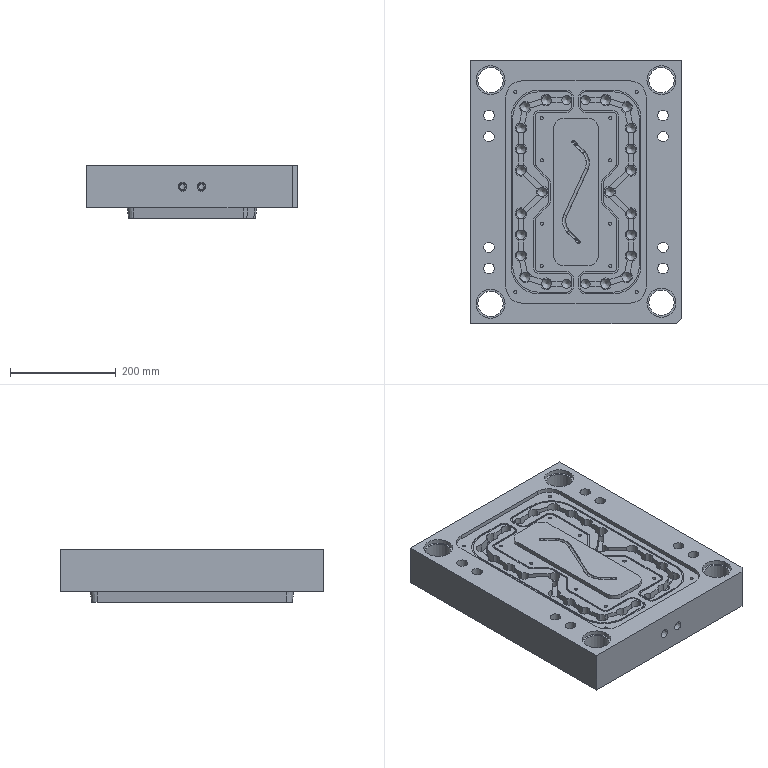Part | STEP file | SL2-MOLD_id54_xmt_txt | 1 solid | 609 faces | box 400 x 500 x 100 mm | volume 12901119 mm3 | cylinder 242 | plane 237 | cone 55 | spline 33 | torus 32 | other 10 | commonest cylinder face diameters 22 x44 20 x28 18 x26 1.219 x16 21 x16 6 x12